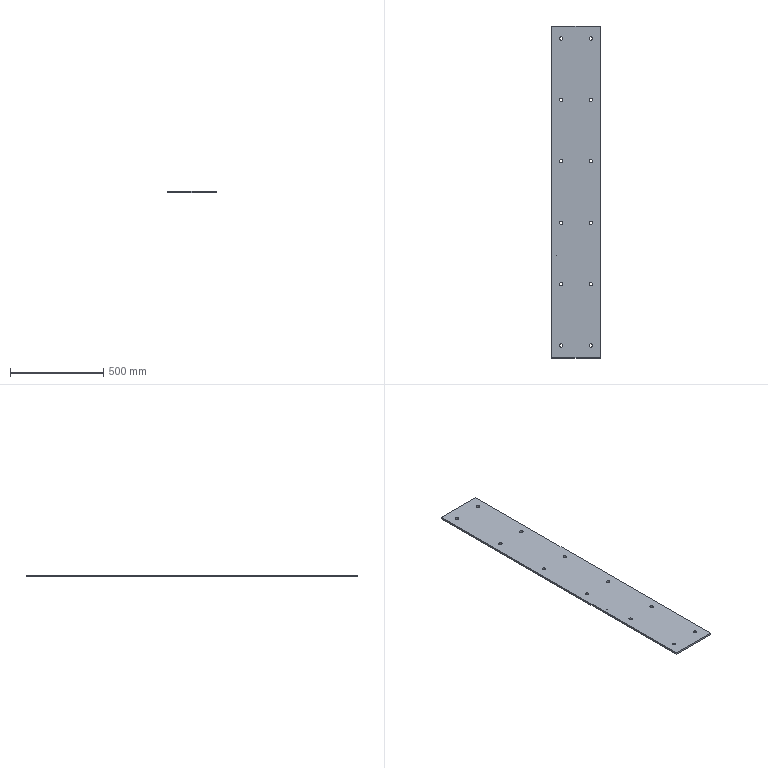Part | STEP file | Rear bottom plate_Default<As machined> | 1 solid | 32 faces | box 260 x 1784 x 10 mm | volume 4607815 mm3 | cylinder 26 | plane 6 | commonest cylinder face diameters 18 x24 2.5 x2